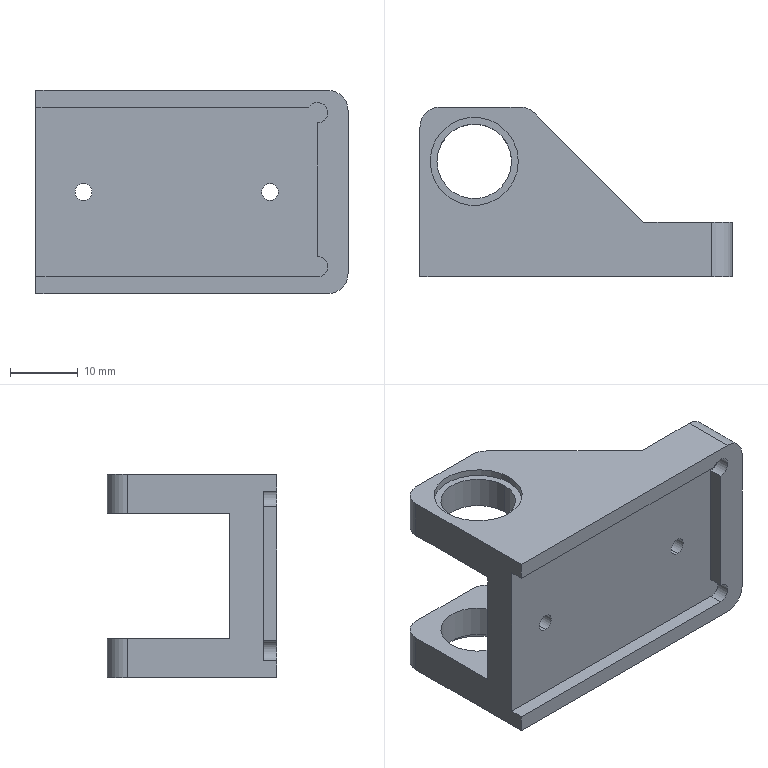Part | NX | features BREP 1 | 1 solid | 43 faces | box 46 x 25 x 30 mm | volume 11465 mm3 | cylinder 22 | plane 21 | commonest cylinder face diameters 6 x6 2.5 x4 11 x4 13 x4 3 x2 8 x2
STEP:
#1=CARTESIAN_POINT('',(26.5,-10.,1.25));
#2=VERTEX_POINT('',#1);
#3=CARTESIAN_POINT('',(26.5,-15.,1.25));
#4=VERTEX_POINT('',#3);
#5=CARTESIAN_POINT('',(26.5,-15.,1.25));
#6=DIRECTION('',(0.,-1.,0.));
#7=VECTOR('',#6,1000.);
#8=LINE('',#5,#7);
#9=EDGE_CURVE('',#2,#4,#8,.T.);
#10=ORIENTED_EDGE('',*,*,#9,.F.);
#11=CARTESIAN_POINT('',(26.5,-10.,-1.25));
#12=VERTEX_POINT('',#11);
#13=CARTESIAN_POINT('',(26.5,-10.,0.));
#14=DIRECTION('',(0.,-1.,0.));
#15=DIRECTION('',(0.,0.,-1.));
#16=AXIS2_PLACEMENT_3D('',#13,#14,#15);
#17=CIRCLE('',#16,1.25);
#18=EDGE_CURVE('',#12,#2,#17,.T.);
#19=ORIENTED_EDGE('',*,*,#18,.F.);
#20=CARTESIAN_POINT('',(26.5,-15.,-1.25));
#21=VERTEX_POINT('',#20);
#22=CARTESIAN_POINT('',(26.5,-15.,-1.25));
#23=DIRECTION('',(0.,-1.,0.));
#24=VECTOR('',#23,1000.);
#25=LINE('',#22,#24);
#26=EDGE_CURVE('',#12,#21,#25,.T.);
#27=ORIENTED_EDGE('',*,*,#26,.T.);
#28=CARTESIAN_POINT('',(26.5,-15.,0.));
#29=DIRECTION('',(0.,-1.,0.));
#30=DIRECTION('',(0.,0.,-1.));
#31=AXIS2_PLACEMENT_3D('',#28,#29,#30);
#32=CIRCLE('',#31,1.25);
#33=EDGE_CURVE('',#21,#4,#32,.T.);
#34=ORIENTED_EDGE('',*,*,#33,.T.);
#35=EDGE_LOOP('',(#10,#19,#27,#34));
#36=FACE_BOUND('',#35,.T.);
#37=CARTESIAN_POINT('',(26.5,-15.,0.));
#38=DIRECTION('',(0.,-1.,0.));
#39=DIRECTION('',(0.,0.,-1.));
#40=AXIS2_PLACEMENT_3D('',#37,#38,#39);
#41=CYLINDRICAL_SURFACE('',#40,1.25);
#42=ADVANCED_FACE('',(#36),#41,.F.);
#43=CARTESIAN_POINT('',(-1.,-10.,1.25));
#44=VERTEX_POINT('',#43);
#45=CARTESIAN_POINT('',(-1.,-15.,1.25));
#46=VERTEX_POINT('',#45);
#47=CARTESIAN_POINT('',(-1.,-15.,1.25));
#48=DIRECTION('',(0.,-1.,0.));
#49=VECTOR('',#48,1000.);
#50=LINE('',#47,#49);
#51=EDGE_CURVE('',#44,#46,#50,.T.);
#52=ORIENTED_EDGE('',*,*,#51,.F.);
#53=CARTESIAN_POINT('',(-1.,-10.,-1.25));
#54=VERTEX_POINT('',#53);
#55=CARTESIAN_POINT('',(-1.,-10.,0.));
#56=DIRECTION('',(0.,-1.,0.));
#57=DIRECTION('',(0.,0.,-1.));
#58=AXIS2_PLACEMENT_3D('',#55,#56,#57);
#59=CIRCLE('',#58,1.25);
#60=EDGE_CURVE('',#54,#44,#59,.T.);
#61=ORIENTED_EDGE('',*,*,#60,.F.);
#62=CARTESIAN_POINT('',(-1.,-15.,-1.25));
#63=VERTEX_POINT('',#62);
#64=CARTESIAN_POINT('',(-1.,-15.,-1.25));
#65=DIRECTION('',(0.,-1.,0.));
#66=VECTOR('',#65,1000.);
#67=LINE('',#64,#66);
#68=EDGE_CURVE('',#54,#63,#67,.T.);
#69=ORIENTED_EDGE('',*,*,#68,.T.);
#70=CARTESIAN_POINT('',(-1.,-15.,0.));
#71=DIRECTION('',(0.,-1.,0.));
#72=DIRECTION('',(0.,0.,-1.));
#73=AXIS2_PLACEMENT_3D('',#70,#71,#72);
#74=CIRCLE('',#73,1.25);
#75=EDGE_CURVE('',#63,#46,#74,.T.);
#76=ORIENTED_EDGE('',*,*,#75,.T.);
#77=EDGE_LOOP('',(#52,#61,#69,#76));
#78=FACE_BOUND('',#77,.T.);
#79=CARTESIAN_POINT('',(-1.,-15.,0.));
#80=DIRECTION('',(0.,-1.,0.));
#81=DIRECTION('',(0.,0.,-1.));
#82=AXIS2_PLACEMENT_3D('',#79,#80,#81);
#83=CYLINDRICAL_SURFACE('',#82,1.25);
#84=ADVANCED_FACE('',(#78),#83,.F.);
#85=CARTESIAN_POINT('',(32.,-13.,4.));
#86=VERTEX_POINT('',#85);
#87=CARTESIAN_POINT('',(32.,-13.,-4.));
#88=VERTEX_POINT('',#87);
#89=CARTESIAN_POINT('',(32.,-13.,0.));
#90=DIRECTION('',(0.,1.,0.));
#91=DIRECTION('',(0.,0.,1.));
#92=AXIS2_PLACEMENT_3D('',#89,#90,#91);
#93=CIRCLE('',#92,4.);
#94=EDGE_CURVE('',#86,#88,#93,.T.);
#95=ORIENTED_EDGE('',*,*,#94,.T.);
#96=CARTESIAN_POINT('',(32.,-13.,0.));
#97=DIRECTION('',(0.,1.,0.));
#98=DIRECTION('',(0.,0.,1.));
#99=AXIS2_PLACEMENT_3D('',#96,#97,#98);
#100=CIRCLE('',#99,4.);
#101=EDGE_CURVE('',#88,#86,#100,.T.);
#102=ORIENTED_EDGE('',*,*,#101,.T.);
#103=EDGE_LOOP('',(#95,#102));
#104=FACE_BOUND('',#103,.T.);
#105=CARTESIAN_POINT('',(32.,-13.,0.));
#106=DIRECTION('',(0.,1.,0.));
#107=DIRECTION('',(0.,0.,1.));
#108=AXIS2_PLACEMENT_3D('',#105,#106,#107);
#109=PLANE('',#108);
#110=ADVANCED_FACE('',(#104),#109,.T.);
#111=CARTESIAN_POINT('',(32.,-10.,-4.));
#112=VERTEX_POINT('',#111);
#113=CARTESIAN_POINT('',(32.,-13.,-4.));
#114=DIRECTION('',(0.,1.,0.));
#115=VECTOR('',#114,1000.);
#116=LINE('',#113,#115);
#117=EDGE_CURVE('',#112,#88,#116,.F.);
#118=ORIENTED_EDGE('',*,*,#117,.T.);
#119=ORIENTED_EDGE('',*,*,#94,.F.);
#120=CARTESIAN_POINT('',(32.,-10.,4.));
#121=VERTEX_POINT('',#120);
#122=CARTESIAN_POINT('',(32.,-13.,4.));
#123=DIRECTION('',(0.,1.,0.));
#124=VECTOR('',#123,1000.);
#125=LINE('',#122,#124);
#126=EDGE_CURVE('',#121,#86,#125,.F.);
#127=ORIENTED_EDGE('',*,*,#126,.F.);
#128=CARTESIAN_POINT('',(32.,-10.,0.));
#129=DIRECTION('',(0.,-1.,0.));
#130=DIRECTION('',(0.,0.,-1.));
#131=AXIS2_PLACEMENT_3D('',#128,#129,#130);
#132=CIRCLE('',#131,4.);
#133=EDGE_CURVE('',#112,#121,#132,.T.);
#134=ORIENTED_EDGE('',*,*,#133,.F.);
#135=EDGE_LOOP('',(#118,#119,#127,#134));
#136=FACE_BOUND('',#135,.T.);
#137=CARTESIAN_POINT('',(32.,-13.,0.));
#138=DIRECTION('',(0.,1.,0.));
#139=DIRECTION('',(0.,0.,1.));
#140=AXIS2_PLACEMENT_3D('',#137,#138,#139);
#141=CYLINDRICAL_SURFACE('',#140,4.);
#142=ADVANCED_FACE('',(#136),#141,.F.);
#143=CARTESIAN_POINT('',(-5.,8.,-9.25));
#144=VERTEX_POINT('',#143);
#145=CARTESIAN_POINT('',(-8.,5.,-9.25));
#146=VERTEX_POINT('',#145);
#147=CARTESIAN_POINT('',(-5.,5.,-9.25));
#148=DIRECTION('',(0.,0.,1.));
#149=DIRECTION('',(0.,1.,0.));
#150=AXIS2_PLACEMENT_3D('',#147,#148,#149);
#151=CIRCLE('',#150,3.);
#152=EDGE_CURVE('',#144,#146,#151,.T.);
#153=ORIENTED_EDGE('',*,*,#152,.F.);
#154=CARTESIAN_POINT('',(-5.,8.,-15.));
#155=VERTEX_POINT('',#154);
#156=CARTESIAN_POINT('',(-5.,8.,15.));
#157=DIRECTION('',(0.,0.,1.));
#158=VECTOR('',#157,1000.);
#159=LINE('',#156,#158);
#160=EDGE_CURVE('',#155,#144,#159,.T.);
#161=ORIENTED_EDGE('',*,*,#160,.F.);
#162=CARTESIAN_POINT('',(-8.,5.,-15.));
#163=VERTEX_POINT('',#162);
#164=CARTESIAN_POINT('',(-5.,5.,-15.));
#165=DIRECTION('',(0.,0.,-1.));
#166=DIRECTION('',(1.,0.,0.));
#167=AXIS2_PLACEMENT_3D('',#164,#165,#166);
#168=CIRCLE('',#167,3.);
#169=EDGE_CURVE('',#163,#155,#168,.T.);
#170=ORIENTED_EDGE('',*,*,#169,.F.);
#171=CARTESIAN_POINT('',(-8.,5.,15.));
#172=DIRECTION('',(0.,0.,-1.));
#173=VECTOR('',#172,1000.);
#174=LINE('',#171,#173);
#175=EDGE_CURVE('',#146,#163,#174,.T.);
#176=ORIENTED_EDGE('',*,*,#175,.F.);
#177=EDGE_LOOP('',(#153,#161,#170,#176));
#178=FACE_BOUND('',#177,.T.);
#179=CARTESIAN_POINT('',(-5.,5.,15.));
#180=DIRECTION('',(0.,0.,-1.));
#181=DIRECTION('',(-1.,0.,0.));
#182=AXIS2_PLACEMENT_3D('',#179,#180,#181);
#183=CYLINDRICAL_SURFACE('',#182,3.);
#184=ADVANCED_FACE('',(#178),#183,.T.);
#185=CARTESIAN_POINT('',(-5.,8.,15.));
#186=VERTEX_POINT('',#185);
#187=CARTESIAN_POINT('',(-8.,5.,15.));
#188=VERTEX_POINT('',#187);
#189=CARTESIAN_POINT('',(-5.,5.,15.));
#190=DIRECTION('',(0.,0.,1.));
#191=DIRECTION('',(1.,0.,0.));
#192=AXIS2_PLACEMENT_3D('',#189,#190,#191);
#193=CIRCLE('',#192,3.);
#194=EDGE_CURVE('',#186,#188,#193,.T.);
#195=ORIENTED_EDGE('',*,*,#194,.F.);
#196=CARTESIAN_POINT('',(-5.,8.,9.25));
#197=VERTEX_POINT('',#196);
#198=CARTESIAN_POINT('',(-5.,8.,15.));
#199=DIRECTION('',(0.,0.,1.));
#200=VECTOR('',#199,1000.);
#201=LINE('',#198,#200);
#202=EDGE_CURVE('',#197,#186,#201,.T.);
#203=ORIENTED_EDGE('',*,*,#202,.F.);
#204=CARTESIAN_POINT('',(-8.,5.,9.25));
#205=VERTEX_POINT('',#204);
#206=CARTESIAN_POINT('',(-5.,5.,9.25));
#207=DIRECTION('',(0.,0.,-1.));
#208=DIRECTION('',(0.,-1.,0.));
#209=AXIS2_PLACEMENT_3D('',#206,#207,#208);
#210=CIRCLE('',#209,3.);
#211=EDGE_CURVE('',#205,#197,#210,.T.);
#212=ORIENTED_EDGE('',*,*,#211,.F.);
#213=CARTESIAN_POINT('',(-8.,5.,15.));
#214=DIRECTION('',(0.,0.,-1.));
#215=VECTOR('',#214,1000.);
#216=LINE('',#213,#215);
#217=EDGE_CURVE('',#188,#205,#216,.T.);
#218=ORIENTED_EDGE('',*,*,#217,.F.);
#219=EDGE_LOOP('',(#195,#203,#212,#218));
#220=FACE_BOUND('',#219,.T.);
#221=CARTESIAN_POINT('',(-5.,5.,15.));
#222=DIRECTION('',(0.,0.,-1.));
#223=DIRECTION('',(-1.,0.,0.));
#224=AXIS2_PLACEMENT_3D('',#221,#222,#223);
#225=CYLINDRICAL_SURFACE('',#224,3.);
#226=ADVANCED_FACE('',(#220),#225,.T.);
#227=CARTESIAN_POINT('',(8.879,7.121,-9.25));
#228=VERTEX_POINT('',#227);
#229=CARTESIAN_POINT('',(6.757,8.,-9.25));
#230=VERTEX_POINT('',#229);
#231=CARTESIAN_POINT('',(6.757,5.,-9.25));
#232=DIRECTION('',(0.,0.,1.));
#233=DIRECTION('',(0.,1.,0.));
#234=AXIS2_PLACEMENT_3D('',#231,#232,#233);
#235=CIRCLE('',#234,3.);
#236=EDGE_CURVE('',#228,#230,#235,.T.);
#237=ORIENTED_EDGE('',*,*,#236,.F.);
#238=CARTESIAN_POINT('',(8.879,7.121,-15.));
#239=VERTEX_POINT('',#238);
#240=CARTESIAN_POINT('',(8.879,7.121,15.));
#241=DIRECTION('',(0.,0.,1.));
#242=VECTOR('',#241,1000.);
#243=LINE('',#240,#242);
#244=EDGE_CURVE('',#239,#228,#243,.T.);
#245=ORIENTED_EDGE('',*,*,#244,.F.);
#246=CARTESIAN_POINT('',(6.757,8.,-15.));
#247=VERTEX_POINT('',#246);
#248=CARTESIAN_POINT('',(6.757,5.,-15.));
#249=DIRECTION('',(0.,0.,-1.));
#250=DIRECTION('',(1.,0.,0.));
#251=AXIS2_PLACEMENT_3D('',#248,#249,#250);
#252=CIRCLE('',#251,3.);
#253=EDGE_CURVE('',#247,#239,#252,.T.);
#254=ORIENTED_EDGE('',*,*,#253,.F.);
#255=CARTESIAN_POINT('',(6.757,8.,15.));
#256=DIRECTION('',(0.,0.,-1.));
#257=VECTOR('',#256,1000.);
#258=LINE('',#255,#257);
#259=EDGE_CURVE('',#230,#247,#258,.T.);
#260=ORIENTED_EDGE('',*,*,#259,.F.);
#261=EDGE_LOOP('',(#237,#245,#254,#260));
#262=FACE_BOUND('',#261,.T.);
#263=CARTESIAN_POINT('',(6.757,5.,15.));
#264=DIRECTION('',(0.,0.,-1.));
#265=DIRECTION('',(-1.,0.,0.));
#266=AXIS2_PLACEMENT_3D('',#263,#264,#265);
#267=CYLINDRICAL_SURFACE('',#266,3.);
#268=ADVANCED_FACE('',(#262),#267,.T.);
#269=CARTESIAN_POINT('',(8.879,7.121,15.));
#270=VERTEX_POINT('',#269);
#271=CARTESIAN_POINT('',(6.757,8.,15.));
#272=VERTEX_POINT('',#271);
#273=CARTESIAN_POINT('',(6.757,5.,15.));
#274=DIRECTION('',(0.,0.,1.));
#275=DIRECTION('',(1.,0.,0.));
#276=AXIS2_PLACEMENT_3D('',#273,#274,#275);
#277=CIRCLE('',#276,3.);
#278=EDGE_CURVE('',#270,#272,#277,.T.);
#279=ORIENTED_EDGE('',*,*,#278,.F.);
#280=CARTESIAN_POINT('',(8.879,7.121,9.25));
#281=VERTEX_POINT('',#280);
#282=CARTESIAN_POINT('',(8.879,7.121,15.));
#283=DIRECTION('',(0.,0.,1.));
#284=VECTOR('',#283,1000.);
#285=LINE('',#282,#284);
#286=EDGE_CURVE('',#281,#270,#285,.T.);
#287=ORIENTED_EDGE('',*,*,#286,.F.);
#288=CARTESIAN_POINT('',(6.757,8.,9.25));
#289=VERTEX_POINT('',#288);
#290=CARTESIAN_POINT('',(6.757,5.,9.25));
#291=DIRECTION('',(0.,0.,-1.));
#292=DIRECTION('',(0.,-1.,0.));
#293=AXIS2_PLACEMENT_3D('',#290,#291,#292);
#294=CIRCLE('',#293,3.);
#295=EDGE_CURVE('',#289,#281,#294,.T.);
#296=ORIENTED_EDGE('',*,*,#295,.F.);
#297=CARTESIAN_POINT('',(6.757,8.,15.));
#298=DIRECTION('',(0.,0.,-1.));
#299=VECTOR('',#298,1000.);
#300=LINE('',#297,#299);
#301=EDGE_CURVE('',#272,#289,#300,.T.);
#302=ORIENTED_EDGE('',*,*,#301,.F.);
#303=EDGE_LOOP('',(#279,#287,#296,#302));
#304=FACE_BOUND('',#303,.T.);
#305=CARTESIAN_POINT('',(6.757,5.,15.));
#306=DIRECTION('',(0.,0.,-1.));
#307=DIRECTION('',(-1.,0.,0.));
#308=AXIS2_PLACEMENT_3D('',#305,#306,#307);
#309=CYLINDRICAL_SURFACE('',#308,3.);
#310=ADVANCED_FACE('',(#304),#309,.T.);
#311=CARTESIAN_POINT('',(38.,-17.,12.));
#312=VERTEX_POINT('',#311);
#313=CARTESIAN_POINT('',(35.,-17.,15.));
#314=VERTEX_POINT('',#313);
#315=CARTESIAN_POINT('',(35.,-17.,12.));
#316=DIRECTION('',(0.,-1.,0.));
#317=DIRECTION('',(0.,0.,1.));
#318=AXIS2_PLACEMENT_3D('',#315,#316,#317);
#319=CIRCLE('',#318,3.);
#320=EDGE_CURVE('',#312,#314,#319,.T.);
#321=ORIENTED_EDGE('',*,*,#320,.F.);
#322=CARTESIAN_POINT('',(38.,-9.,12.));
#323=VERTEX_POINT('',#322);
#324=CARTESIAN_POINT('',(38.,-17.,12.));
#325=DIRECTION('',(0.,-1.,0.));
#326=VECTOR('',#325,1000.);
#327=LINE('',#324,#326);
#328=EDGE_CURVE('',#323,#312,#327,.T.);
#329=ORIENTED_EDGE('',*,*,#328,.F.);
#330=CARTESIAN_POINT('',(35.,-9.,15.));
#331=VERTEX_POINT('',#330);
#332=CARTESIAN_POINT('',(35.,-9.,12.));
#333=DIRECTION('',(0.,1.,0.));
#334=DIRECTION('',(0.,0.,-1.));
#335=AXIS2_PLACEMENT_3D('',#332,#333,#334);
#336=CIRCLE('',#335,3.);
#337=EDGE_CURVE('',#331,#323,#336,.T.);
#338=ORIENTED_EDGE('',*,*,#337,.F.);
#339=CARTESIAN_POINT('',(35.,-9.,15.));
#340=DIRECTION('',(0.,1.,0.));
#341=VECTOR('',#340,1000.);
#342=LINE('',#339,#341);
#343=EDGE_CURVE('',#314,#331,#342,.T.);
#344=ORIENTED_EDGE('',*,*,#343,.F.);
#345=EDGE_LOOP('',(#321,#329,#338,#344));
#346=FACE_BOUND('',#345,.T.);
#347=CARTESIAN_POINT('',(35.,0.,12.));
#348=DIRECTION('',(0.,-1.,0.));
#349=DIRECTION('',(0.,0.,-1.));
#350=AXIS2_PLACEMENT_3D('',#347,#348,#349);
#351=CYLINDRICAL_SURFACE('',#350,3.);
#352=ADVANCED_FACE('',(#346),#351,.T.);
#353=CARTESIAN_POINT('',(35.,-17.,-15.));
#354=VERTEX_POINT('',#353);
#355=CARTESIAN_POINT('',(38.,-17.,-12.));
#356=VERTEX_POINT('',#355);
#357=CARTESIAN_POINT('',(35.,-17.,-12.));
#358=DIRECTION('',(0.,-1.,0.));
#359=DIRECTION('',(0.,0.,1.));
#360=AXIS2_PLACEMENT_3D('',#357,#358,#359);
#361=CIRCLE('',#360,3.);
#362=EDGE_CURVE('',#354,#356,#361,.T.);
#363=ORIENTED_EDGE('',*,*,#362,.F.);
#364=CARTESIAN_POINT('',(35.,-9.,-15.));
#365=VERTEX_POINT('',#364);
#366=CARTESIAN_POINT('',(35.,0.,-15.));
#367=DIRECTION('',(0.,-1.,0.));
#368=VECTOR('',#367,1000.);
#369=LINE('',#366,#368);
#370=EDGE_CURVE('',#365,#354,#369,.T.);
#371=ORIENTED_EDGE('',*,*,#370,.F.);
#372=CARTESIAN_POINT('',(38.,-9.,-12.));
#373=VERTEX_POINT('',#372);
#374=CARTESIAN_POINT('',(35.,-9.,-12.));
#375=DIRECTION('',(0.,1.,0.));
#376=DIRECTION('',(0.,0.,-1.));
#377=AXIS2_PLACEMENT_3D('',#374,#375,#376);
#378=CIRCLE('',#377,3.);
#379=EDGE_CURVE('',#373,#365,#378,.T.);
#380=ORIENTED_EDGE('',*,*,#379,.F.);
#381=CARTESIAN_POINT('',(38.,-9.,-12.));
#382=DIRECTION('',(0.,1.,0.));
#383=VECTOR('',#382,1000.);
#384=LINE('',#381,#383);
#385=EDGE_CURVE('',#356,#373,#384,.T.);
#386=ORIENTED_EDGE('',*,*,#385,.F.);
#387=EDGE_LOOP('',(#363,#371,#380,#386));
#388=FACE_BOUND('',#387,.T.);
#389=CARTESIAN_POINT('',(35.,-9.,-12.));
#390=DIRECTION('',(0.,1.,0.));
#391=DIRECTION('',(0.,0.,1.));
#392=AXIS2_PLACEMENT_3D('',#389,#390,#391);
#393=CYLINDRICAL_SURFACE('',#392,3.);
#394=ADVANCED_FACE('',(#388),#393,.T.);
#395=CARTESIAN_POINT('',(-8.,-15.,12.5));
#396=VERTEX_POINT('',#395);
#397=CARTESIAN_POINT('',(-8.,-15.,-12.5));
#398=VERTEX_POINT('',#397);
#399=CARTESIAN_POINT('',(-8.,-15.,12.5));
#400=DIRECTION('',(0.,0.,-1.));
#401=VECTOR('',#400,1000.);
#402=LINE('',#399,#401);
#403=EDGE_CURVE('',#396,#398,#402,.T.);
#404=ORIENTED_EDGE('',*,*,#403,.T.);
#405=CARTESIAN_POINT('',(33.5,-15.,-12.5));
#406=VERTEX_POINT('',#405);
#407=CARTESIAN_POINT('',(33.5,-15.,-12.5));
#408=DIRECTION('',(1.,0.,0.));
#409=VECTOR('',#408,1000.);
#410=LINE('',#407,#409);
#411=EDGE_CURVE('',#398,#406,#410,.T.);
#412=ORIENTED_EDGE('',*,*,#411,.T.);
#413=CARTESIAN_POINT('',(33.5,-15.,-9.5));
#414=VERTEX_POINT('',#413);
#415=CARTESIAN_POINT('',(33.5,-15.,-11.));
#416=DIRECTION('',(0.,-1.,0.));
#417=DIRECTION('',(0.,0.,-1.));
#418=AXIS2_PLACEMENT_3D('',#415,#416,#417);
#419=CIRCLE('',#418,1.5);
#420=EDGE_CURVE('',#406,#414,#419,.T.);
#421=ORIENTED_EDGE('',*,*,#420,.T.);
#422=CARTESIAN_POINT('',(33.5,-15.,10.202));
#423=VERTEX_POINT('',#422);
#424=CARTESIAN_POINT('',(33.5,-15.,10.202));
#425=DIRECTION('',(0.,0.,1.));
#426=VECTOR('',#425,1000.);
#427=LINE('',#424,#426);
#428=EDGE_CURVE('',#414,#423,#427,.T.);
#429=ORIENTED_EDGE('',*,*,#428,.T.);
#430=CARTESIAN_POINT('',(32.23,-15.,12.5));
#431=VERTEX_POINT('',#430);
#432=CARTESIAN_POINT('',(33.5,-15.,11.702));
#433=DIRECTION('',(0.,-1.,0.));
#434=DIRECTION('',(0.,0.,-1.));
#435=AXIS2_PLACEMENT_3D('',#432,#433,#434);
#436=CIRCLE('',#435,1.5);
#437=EDGE_CURVE('',#423,#431,#436,.T.);
#438=ORIENTED_EDGE('',*,*,#437,.T.);
#439=CARTESIAN_POINT('',(32.23,-15.,12.5));
#440=DIRECTION('',(-1.,0.,0.));
#441=VECTOR('',#440,1000.);
#442=LINE('',#439,#441);
#443=EDGE_CURVE('',#431,#396,#442,.T.);
#444=ORIENTED_EDGE('',*,*,#443,.T.);
#445=EDGE_LOOP('',(#404,#412,#421,#429,#438,#444));
#446=FACE_BOUND('',#445,.T.);
#447=ORIENTED_EDGE('',*,*,#75,.F.);
#448=CARTESIAN_POINT('',(-1.,-15.,0.));
#449=DIRECTION('',(0.,-1.,0.));
#450=DIRECTION('',(0.,0.,-1.));
#451=AXIS2_PLACEMENT_3D('',#448,#449,#450);
#452=CIRCLE('',#451,1.25);
#453=EDGE_CURVE('',#46,#63,#452,.T.);
#454=ORIENTED_EDGE('',*,*,#453,.F.);
#455=EDGE_LOOP('',(#447,#454));
#456=FACE_BOUND('',#455,.T.);
#457=ORIENTED_EDGE('',*,*,#33,.F.);
#458=CARTESIAN_POINT('',(26.5,-15.,0.));
#459=DIRECTION('',(0.,-1.,0.));
#460=DIRECTION('',(0.,0.,-1.));
#461=AXIS2_PLACEMENT_3D('',#458,#459,#460);
#462=CIRCLE('',#461,1.25);
#463=EDGE_CURVE('',#4,#21,#462,.T.);
#464=ORIENTED_EDGE('',*,*,#463,.F.);
#465=EDGE_LOOP('',(#457,#464));
#466=FACE_BOUND('',#465,.T.);
#467=CARTESIAN_POINT('',(33.5,-15.,-11.));
#468=DIRECTION('',(0.,-1.,0.));
#469=DIRECTION('',(0.,0.,-1.));
#470=AXIS2_PLACEMENT_3D('',#467,#468,#469);
#471=PLANE('',#470);
#472=ADVANCED_FACE('',(#446,#456,#466),#471,.T.);
#473=CARTESIAN_POINT('',(-8.,-17.,-12.5));
#474=VERTEX_POINT('',#473);
#475=CARTESIAN_POINT('',(33.5,-17.,-12.5));
#476=VERTEX_POINT('',#475);
#477=CARTESIAN_POINT('',(33.5,-17.,-12.5));
#478=DIRECTION('',(1.,0.,0.));
#479=VECTOR('',#478,1000.);
#480=LINE('',#477,#479);
#481=EDGE_CURVE('',#474,#476,#480,.T.);
#482=ORIENTED_EDGE('',*,*,#481,.T.);
#483=CARTESIAN_POINT('',(33.5,-15.,-12.5));
#484=DIRECTION('',(0.,-1.,0.));
#485=VECTOR('',#484,1000.);
#486=LINE('',#483,#485);
#487=EDGE_CURVE('',#406,#476,#486,.T.);
#488=ORIENTED_EDGE('',*,*,#487,.F.);
#489=ORIENTED_EDGE('',*,*,#411,.F.);
#490=CARTESIAN_POINT('',(-8.,-15.,-12.5));
#491=DIRECTION('',(0.,-1.,0.));
#492=VECTOR('',#491,1000.);
#493=LINE('',#490,#492);
#494=EDGE_CURVE('',#398,#474,#493,.T.);
#495=ORIENTED_EDGE('',*,*,#494,.T.);
#496=EDGE_LOOP('',(#482,#488,#489,#495));
#497=FACE_BOUND('',#496,.T.);
#498=CARTESIAN_POINT('',(33.5,-15.,-12.5));
#499=DIRECTION('',(0.,0.,-1.));
#500=DIRECTION('',(-1.,0.,0.));
#501=AXIS2_PLACEMENT_3D('',#498,#499,#500);
#502=PLANE('',#501);
#503=ADVANCED_FACE('',(#497),#502,.F.);
#504=CARTESIAN_POINT('',(33.5,-17.,-9.5));
#505=VERTEX_POINT('',#504);
#506=CARTESIAN_POINT('',(33.5,-17.,-11.));
#507=DIRECTION('',(0.,-1.,0.));
#508=DIRECTION('',(0.,0.,-1.));
#509=AXIS2_PLACEMENT_3D('',#506,#507,#508);
#510=CIRCLE('',#509,1.5);
#511=EDGE_CURVE('',#476,#505,#510,.T.);
#512=ORIENTED_EDGE('',*,*,#511,.T.);
#513=CARTESIAN_POINT('',(33.5,-15.,-9.5));
#514=DIRECTION('',(0.,-1.,0.));
#515=VECTOR('',#514,1000.);
#516=LINE('',#513,#515);
#517=EDGE_CURVE('',#414,#505,#516,.T.);
#518=ORIENTED_EDGE('',*,*,#517,.F.);
#519=ORIENTED_EDGE('',*,*,#420,.F.);
#520=ORIENTED_EDGE('',*,*,#487,.T.);
#521=EDGE_LOOP('',(#512,#518,#519,#520));
#522=FACE_BOUND('',#521,.T.);
#523=CARTESIAN_POINT('',(33.5,-15.,-11.));
#524=DIRECTION('',(0.,-1.,0.));
#525=DIRECTION('',(0.,0.,-1.));
#526=AXIS2_PLACEMENT_3D('',#523,#524,#525);
#527=CYLINDRICAL_SURFACE('',#526,1.5);
#528=ADVANCED_FACE('',(#522),#527,.F.);
#529=CARTESIAN_POINT('',(33.5,-17.,10.202));
#530=VERTEX_POINT('',#529);
#531=CARTESIAN_POINT('',(33.5,-17.,10.202));
#532=DIRECTION('',(0.,0.,1.));
#533=VECTOR('',#532,1000.);
#534=LINE('',#531,#533);
#535=EDGE_CURVE('',#505,#530,#534,.T.);
#536=ORIENTED_EDGE('',*,*,#535,.T.);
#537=CARTESIAN_POINT('',(33.5,-15.,10.202));
#538=DIRECTION('',(0.,-1.,0.));
#539=VECTOR('',#538,1000.);
#540=LINE('',#537,#539);
#541=EDGE_CURVE('',#423,#530,#540,.T.);
#542=ORIENTED_EDGE('',*,*,#541,.F.);
#543=ORIENTED_EDGE('',*,*,#428,.F.);
#544=ORIENTED_EDGE('',*,*,#517,.T.);
#545=EDGE_LOOP('',(#536,#542,#543,#544));
#546=FACE_BOUND('',#545,.T.);
#547=CARTESIAN_POINT('',(33.5,-15.,10.202));
#548=DIRECTION('',(1.,0.,0.));
#549=DIRECTION('',(0.,0.,-1.));
#550=AXIS2_PLACEMENT_3D('',#547,#548,#549);
#551=PLANE('',#550);
#552=ADVANCED_FACE('',(#546),#551,.F.);
#553=CARTESIAN_POINT('',(32.23,-17.,12.5));
#554=VERTEX_POINT('',#553);
#555=CARTESIAN_POINT('',(33.5,-17.,11.702));
#556=DIRECTION('',(0.,-1.,0.));
#557=DIRECTION('',(0.,0.,-1.));
#558=AXIS2_PLACEMENT_3D('',#555,#556,#557);
#559=CIRCLE('',#558,1.5);
#560=EDGE_CURVE('',#530,#554,#559,.T.);
#561=ORIENTED_EDGE('',*,*,#560,.T.);
#562=CARTESIAN_POINT('',(32.23,-15.,12.5));
#563=DIRECTION('',(0.,-1.,0.));
#564=VECTOR('',#563,1000.);
#565=LINE('',#562,#564);
#566=EDGE_CURVE('',#431,#554,#565,.T.);
#567=ORIENTED_EDGE('',*,*,#566,.F.);
#568=ORIENTED_EDGE('',*,*,#437,.F.);
#569=ORIENTED_EDGE('',*,*,#541,.T.);
#570=EDGE_LOOP('',(#561,#567,#568,#569));
#571=FACE_BOUND('',#570,.T.);
#572=CARTESIAN_POINT('',(33.5,-15.,11.702));
#573=DIRECTION('',(0.,-1.,0.));
#574=DIRECTION('',(0.,0.,-1.));
#575=AXIS2_PLACEMENT_3D('',#572,#573,#574);
#576=CYLINDRICAL_SURFACE('',#575,1.5);
#577=ADVANCED_FACE('',(#571),#576,.F.);
#578=CARTESIAN_POINT('',(-8.,-17.,12.5));
#579=VERTEX_POINT('',#578);
#580=CARTESIAN_POINT('',(32.23,-17.,12.5));
#581=DIRECTION('',(-1.,0.,0.));
#582=VECTOR('',#581,1000.);
#583=LINE('',#580,#582);
#584=EDGE_CURVE('',#554,#579,#583,.T.);
#585=ORIENTED_EDGE('',*,*,#584,.T.);
#586=CARTESIAN_POINT('',(-8.,-15.,12.5));
#587=DIRECTION('',(0.,-1.,0.));
#588=VECTOR('',#587,1000.);
#589=LINE('',#586,#588);
#590=EDGE_CURVE('',#396,#579,#589,.T.);
#591=ORIENTED_EDGE('',*,*,#590,.F.);
#592=ORIENTED_EDGE('',*,*,#443,.F.);
#593=ORIENTED_EDGE('',*,*,#566,.T.);
#594=EDGE_LOOP('',(#585,#591,#592,#593));
#595=FACE_BOUND('',#594,.T.);
#596=CARTESIAN_POINT('',(32.23,-15.,12.5));
#597=DIRECTION('',(0.,0.,1.));
#598=DIRECTION('',(1.,0.,0.));
#599=AXIS2_PLACEMENT_3D('',#596,#597,#598);
#600=PLANE('',#599);
#601=ADVANCED_FACE('',(#595),#600,.F.);
#602=CARTESIAN_POINT('',(-6.5,0.,-14.));
#603=VERTEX_POINT('',#602);
#604=CARTESIAN_POINT('',(6.5,0.,-14.));
#605=VERTEX_POINT('',#604);
#606=CARTESIAN_POINT('',(0.,0.,-14.));
#607=DIRECTION('',(0.,0.,-1.));
#608=DIRECTION('',(-1.,0.,0.));
#609=AXIS2_PLACEMENT_3D('',#606,#607,#608);
#610=CIRCLE('',#609,6.5);
#611=EDGE_CURVE('',#603,#605,#610,.T.);
#612=ORIENTED_EDGE('',*,*,#611,.T.);
#613=CARTESIAN_POINT('',(0.,0.,-14.));
#614=DIRECTION('',(0.,0.,-1.));
#615=DIRECTION('',(-1.,0.,0.));
#616=AXIS2_PLACEMENT_3D('',#613,#614,#615);
#617=CIRCLE('',#616,6.5);
#618=EDGE_CURVE('',#605,#603,#617,.T.);
#619=ORIENTED_EDGE('',*,*,#618,.T.);
#620=EDGE_LOOP('',(#612,#619));
#621=FACE_BOUND('',#620,.T.);
#622=CARTESIAN_POINT('',(-5.5,0.,-14.));
#623=VERTEX_POINT('',#622);
#624=CARTESIAN_POINT('',(5.5,0.,-14.));
#625=VERTEX_POINT('',#624);
#626=CARTESIAN_POINT('',(0.,0.,-14.));
#627=DIRECTION('',(0.,0.,-1.));
#628=DIRECTION('',(-1.,0.,0.));
#629=AXIS2_PLACEMENT_3D('',#626,#627,#628);
#630=CIRCLE('',#629,5.5);
#631=EDGE_CURVE('',#623,#625,#630,.T.);
#632=ORIENTED_EDGE('',*,*,#631,.F.);
#633=CARTESIAN_POINT('',(0.,0.,-14.));
#634=DIRECTION('',(0.,0.,-1.));
#635=DIRECTION('',(-1.,0.,0.));
#636=AXIS2_PLACEMENT_3D('',#633,#634,#635);
#637=CIRCLE('',#636,5.5);
#638=EDGE_CURVE('',#625,#623,#637,.T.);
#639=ORIENTED_EDGE('',*,*,#638,.F.);
#640=EDGE_LOOP('',(#632,#639));
#641=FACE_BOUND('',#640,.T.);
#642=CARTESIAN_POINT('',(0.,0.,-14.));
#643=DIRECTION('',(0.,0.,-1.));
#644=DIRECTION('',(-1.,0.,0.));
#645=AXIS2_PLACEMENT_3D('',#642,#643,#644);
#646=PLANE('',#645);
#647=ADVANCED_FACE('',(#621,#641),#646,.T.);
#648=CARTESIAN_POINT('',(6.5,0.,-15.));
#649=VERTEX_POINT('',#648);
#650=CARTESIAN_POINT('',(6.5,0.,-14.));
#651=DIRECTION('',(0.,0.,-1.));
#652=VECTOR('',#651,1000.);
#653=LINE('',#650,#652);
#654=EDGE_CURVE('',#605,#649,#653,.T.);
#655=ORIENTED_EDGE('',*,*,#654,.F.);
#656=ORIENTED_EDGE('',*,*,#611,.F.);
#657=CARTESIAN_POINT('',(-6.5,0.,-15.));
#658=VERTEX_POINT('',#657);
#659=CARTESIAN_POINT('',(-6.5,0.,-14.));
#660=DIRECTION('',(0.,0.,-1.));
#661=VECTOR('',#660,1000.);
#662=LINE('',#659,#661);
#663=EDGE_CURVE('',#603,#658,#662,.T.);
#664=ORIENTED_EDGE('',*,*,#663,.T.);
#665=CARTESIAN_POINT('',(0.,0.,-15.));
#666=DIRECTION('',(0.,0.,-1.));
#667=DIRECTION('',(-1.,0.,0.));
#668=AXIS2_PLACEMENT_3D('',#665,#666,#667);
#669=CIRCLE('',#668,6.5);
#670=EDGE_CURVE('',#658,#649,#669,.T.);
#671=ORIENTED_EDGE('',*,*,#670,.T.);
#672=EDGE_LOOP('',(#655,#656,#664,#671));
#673=FACE_BOUND('',#672,.T.);
#674=CARTESIAN_POINT('',(0.,0.,-14.));
#675=DIRECTION('',(0.,0.,-1.));
#676=DIRECTION('',(-1.,0.,0.));
#677=AXIS2_PLACEMENT_3D('',#674,#675,#676);
#678=CYLINDRICAL_SURFACE('',#677,6.5);
#679=ADVANCED_FACE('',(#673),#678,.F.);
#680=CARTESIAN_POINT('',(6.5,0.,14.));
#681=VERTEX_POINT('',#680);
#682=CARTESIAN_POINT('',(-6.5,0.,14.));
#683=VERTEX_POINT('',#682);
#684=CARTESIAN_POINT('',(0.,0.,14.));
#685=DIRECTION('',(0.,0.,1.));
#686=DIRECTION('',(1.,0.,0.));
#687=AXIS2_PLACEMENT_3D('',#684,#685,#686);
#688=CIRCLE('',#687,6.5);
#689=EDGE_CURVE('',#681,#683,#688,.T.);
#690=ORIENTED_EDGE('',*,*,#689,.T.);
#691=CARTESIAN_POINT('',(0.,0.,14.));
#692=DIRECTION('',(0.,0.,1.));
#693=DIRECTION('',(1.,0.,0.));
#694=AXIS2_PLACEMENT_3D('',#691,#692,#693);
#695=CIRCLE('',#694,6.5);
#696=EDGE_CURVE('',#683,#681,#695,.T.);
#697=ORIENTED_EDGE('',*,*,#696,.T.);
#698=EDGE_LOOP('',(#690,#697));
#699=FACE_BOUND('',#698,.T.);
#700=CARTESIAN_POINT('',(-5.5,0.,14.));
#701=VERTEX_POINT('',#700);
#702=CARTESIAN_POINT('',(5.5,0.,14.));
#703=VERTEX_POINT('',#702);
#704=CARTESIAN_POINT('',(0.,0.,14.));
#705=DIRECTION('',(0.,0.,1.));
#706=DIRECTION('',(1.,0.,0.));
#707=AXIS2_PLACEMENT_3D('',#704,#705,#706);
#708=CIRCLE('',#707,5.5);
#709=EDGE_CURVE('',#701,#703,#708,.T.);
#710=ORIENTED_EDGE('',*,*,#709,.F.);
#711=CARTESIAN_POINT('',(0.,0.,14.));
#712=DIRECTION('',(0.,0.,1.));
#713=DIRECTION('',(1.,0.,0.));
#714=AXIS2_PLACEMENT_3D('',#711,#712,#713);
#715=CIRCLE('',#714,5.5);
#716=EDGE_CURVE('',#703,#701,#715,.T.);
#717=ORIENTED_EDGE('',*,*,#716,.F.);
#718=EDGE_LOOP('',(#710,#717));
#719=FACE_BOUND('',#718,.T.);
#720=CARTESIAN_POINT('',(0.,0.,14.));
#721=DIRECTION('',(0.,0.,1.));
#722=DIRECTION('',(1.,0.,0.));
#723=AXIS2_PLACEMENT_3D('',#720,#721,#722);
#724=PLANE('',#723);
#725=ADVANCED_FACE('',(#699,#719),#724,.T.);
#726=CARTESIAN_POINT('',(-6.5,0.,15.));
#727=VERTEX_POINT('',#726);
#728=CARTESIAN_POINT('',(-6.5,0.,14.));
#729=DIRECTION('',(0.,0.,1.));
#730=VECTOR('',#729,1000.);
#731=LINE('',#728,#730);
#732=EDGE_CURVE('',#727,#683,#731,.F.);
#733=ORIENTED_EDGE('',*,*,#732,.T.);
#734=ORIENTED_EDGE('',*,*,#689,.F.);
#735=CARTESIAN_POINT('',(6.5,0.,15.));
#736=VERTEX_POINT('',#735);
#737=CARTESIAN_POINT('',(6.5,0.,14.));
#738=DIRECTION('',(0.,0.,1.));
#739=VECTOR('',#738,1000.);
#740=LINE('',#737,#739);
#741=EDGE_CURVE('',#736,#681,#740,.F.);
#742=ORIENTED_EDGE('',*,*,#741,.F.);
#743=CARTESIAN_POINT('',(0.,0.,15.));
#744=DIRECTION('',(0.,0.,1.));
#745=DIRECTION('',(1.,0.,0.));
#746=AXIS2_PLACEMENT_3D('',#743,#744,#745);
#747=CIRCLE('',#746,6.5);
#748=EDGE_CURVE('',#736,#727,#747,.T.);
#749=ORIENTED_EDGE('',*,*,#748,.T.);
#750=EDGE_LOOP('',(#733,#734,#742,#749));
#751=FACE_BOUND('',#750,.T.);
#752=CARTESIAN_POINT('',(0.,0.,14.));
#753=DIRECTION('',(0.,0.,1.));
#754=DIRECTION('',(1.,0.,0.));
#755=AXIS2_PLACEMENT_3D('',#752,#753,#754);
#756=CYLINDRICAL_SURFACE('',#755,6.5);
#757=ADVANCED_FACE('',(#751),#756,.F.);
#758=CARTESIAN_POINT('',(-8.,-10.,-9.25));
#759=VERTEX_POINT('',#758);
#760=CARTESIAN_POINT('',(-8.,-10.,9.25));
#761=VERTEX_POINT('',#760);
#762=CARTESIAN_POINT('',(-8.,-10.,-9.25));
#763=DIRECTION('',(0.,0.,1.));
#764=VECTOR('',#763,1000.);
#765=LINE('',#762,#764);
#766=EDGE_CURVE('',#759,#761,#765,.T.);
#767=ORIENTED_EDGE('',*,*,#766,.T.);
#768=CARTESIAN_POINT('',(38.,-10.,9.25));
#769=VERTEX_POINT('',#768);
#770=CARTESIAN_POINT('',(38.,-10.,9.25));
#771=DIRECTION('',(-1.,0.,0.));
#772=VECTOR('',#771,1000.);
#773=LINE('',#770,#772);
#774=EDGE_CURVE('',#769,#761,#773,.T.);
#775=ORIENTED_EDGE('',*,*,#774,.F.);
#776=CARTESIAN_POINT('',(38.,-10.,-9.25));
#777=VERTEX_POINT('',#776);
#778=CARTESIAN_POINT('',(38.,-10.,-9.25));
#779=DIRECTION('',(0.,0.,1.));
#780=VECTOR('',#779,1000.);
#781=LINE('',#778,#780);
#782=EDGE_CURVE('',#777,#769,#781,.T.);
#783=ORIENTED_EDGE('',*,*,#782,.F.);
#784=CARTESIAN_POINT('',(38.,-10.,-9.25));
#785=DIRECTION('',(-1.,0.,0.));
#786=VECTOR('',#785,1000.);
#787=LINE('',#784,#786);
#788=EDGE_CURVE('',#777,#759,#787,.T.);
#789=ORIENTED_EDGE('',*,*,#788,.T.);
#790=EDGE_LOOP('',(#767,#775,#783,#789));
#791=FACE_BOUND('',#790,.T.);
#792=CARTESIAN_POINT('',(32.,-10.,0.));
#793=DIRECTION('',(0.,-1.,0.));
#794=DIRECTION('',(0.,0.,-1.));
#795=AXIS2_PLACEMENT_3D('',#792,#793,#794);
#796=CIRCLE('',#795,4.);
#797=EDGE_CURVE('',#121,#112,#796,.T.);
#798=ORIENTED_EDGE('',*,*,#797,.T.);
#799=ORIENTED_EDGE('',*,*,#133,.T.);
#800=EDGE_LOOP('',(#798,#799));
#801=FACE_BOUND('',#800,.T.);
#802=ORIENTED_EDGE('',*,*,#60,.T.);
#803=CARTESIAN_POINT('',(-1.,-10.,0.));
#804=DIRECTION('',(0.,-1.,0.));
#805=DIRECTION('',(0.,0.,-1.));
#806=AXIS2_PLACEMENT_3D('',#803,#804,#805);
#807=CIRCLE('',#806,1.25);
#808=EDGE_CURVE('',#44,#54,#807,.T.);
#809=ORIENTED_EDGE('',*,*,#808,.T.);
#810=EDGE_LOOP('',(#802,#809));
#811=FACE_BOUND('',#810,.T.);
#812=ORIENTED_EDGE('',*,*,#18,.T.);
#813=CARTESIAN_POINT('',(26.5,-10.,0.));
#814=DIRECTION('',(0.,-1.,0.));
#815=DIRECTION('',(0.,0.,-1.));
#816=AXIS2_PLACEMENT_3D('',#813,#814,#815);
#817=CIRCLE('',#816,1.25);
#818=EDGE_CURVE('',#2,#12,#817,.T.);
#819=ORIENTED_EDGE('',*,*,#818,.T.);
#820=EDGE_LOOP('',(#812,#819));
#821=FACE_BOUND('',#820,.T.);
#822=CARTESIAN_POINT('',(38.,-10.,-9.25));
#823=DIRECTION('',(0.,-1.,0.));
#824=DIRECTION('',(0.,0.,-1.));
#825=AXIS2_PLACEMENT_3D('',#822,#823,#824);
#826=PLANE('',#825);
#827=ADVANCED_FACE('',(#791,#801,#811,#821),#826,.F.);
#828=CARTESIAN_POINT('',(25.,-9.,-9.25));
#829=VERTEX_POINT('',#828);
#830=CARTESIAN_POINT('',(8.,8.,-9.25));
#831=DIRECTION('',(0.7071,-0.7071,0.));
#832=VECTOR('',#831,1000.);
#833=LINE('',#830,#832);
#834=EDGE_CURVE('',#228,#829,#833,.T.);
#835=ORIENTED_EDGE('',*,*,#834,.F.);
#836=ORIENTED_EDGE('',*,*,#236,.T.);
#837=CARTESIAN_POINT('',(-8.,8.,-9.25));
#838=DIRECTION('',(1.,0.,0.));
#839=VECTOR('',#838,1000.);
#840=LINE('',#837,#839);
#841=EDGE_CURVE('',#144,#230,#840,.T.);
#842=ORIENTED_EDGE('',*,*,#841,.F.);
#843=ORIENTED_EDGE('',*,*,#152,.T.);
#844=CARTESIAN_POINT('',(-8.,26.,-9.25));
#845=DIRECTION('',(0.,-1.,0.));
#846=VECTOR('',#845,1000.);
#847=LINE('',#844,#846);
#848=EDGE_CURVE('',#146,#759,#847,.T.);
#849=ORIENTED_EDGE('',*,*,#848,.T.);
#850=ORIENTED_EDGE('',*,*,#788,.F.);
#851=CARTESIAN_POINT('',(38.,-9.,-9.25));
#852=VERTEX_POINT('',#851);
#853=CARTESIAN_POINT('',(38.,26.,-9.25));
#854=DIRECTION('',(0.,-1.,0.));
#855=VECTOR('',#854,1000.);
#856=LINE('',#853,#855);
#857=EDGE_CURVE('',#852,#777,#856,.T.);
#858=ORIENTED_EDGE('',*,*,#857,.F.);
#859=CARTESIAN_POINT('',(25.,-9.,-9.25));
#860=DIRECTION('',(1.,0.,0.));
#861=VECTOR('',#860,1000.);
#862=LINE('',#859,#861);
#863=EDGE_CURVE('',#829,#852,#862,.T.);
#864=ORIENTED_EDGE('',*,*,#863,.F.);
#865=EDGE_LOOP('',(#835,#836,#842,#843,#849,#850,#858,#864));
#866=FACE_BOUND('',#865,.T.);
#867=CARTESIAN_POINT('',(-5.5,0.,-9.25));
#868=VERTEX_POINT('',#867);
#869=CARTESIAN_POINT('',(5.5,0.,-9.25));
#870=VERTEX_POINT('',#869);
#871=CARTESIAN_POINT('',(0.,0.,-9.25));
#872=DIRECTION('',(0.,0.,-1.));
#873=DIRECTION('',(0.,1.,0.));
#874=AXIS2_PLACEMENT_3D('',#871,#872,#873);
#875=CIRCLE('',#874,5.5);
#876=EDGE_CURVE('',#868,#870,#875,.T.);
#877=ORIENTED_EDGE('',*,*,#876,.T.);
#878=CARTESIAN_POINT('',(0.,0.,-9.25));
#879=DIRECTION('',(0.,0.,-1.));
#880=DIRECTION('',(0.,1.,0.));
#881=AXIS2_PLACEMENT_3D('',#878,#879,#880);
#882=CIRCLE('',#881,5.5);
#883=EDGE_CURVE('',#870,#868,#882,.T.);
#884=ORIENTED_EDGE('',*,*,#883,.T.);
#885=EDGE_LOOP('',(#877,#884));
#886=FACE_BOUND('',#885,.T.);
#887=CARTESIAN_POINT('',(38.,26.,-9.25));
#888=DIRECTION('',(0.,0.,-1.));
#889=DIRECTION('',(0.,1.,0.));
#890=AXIS2_PLACEMENT_3D('',#887,#888,#889);
#891=PLANE('',#890);
#892=ADVANCED_FACE('',(#866,#886),#891,.F.);
#893=CARTESIAN_POINT('',(-8.,8.,9.25));
#894=DIRECTION('',(-1.,0.,0.));
#895=VECTOR('',#894,1000.);
#896=LINE('',#893,#895);
#897=EDGE_CURVE('',#289,#197,#896,.T.);
#898=ORIENTED_EDGE('',*,*,#897,.F.);
#899=ORIENTED_EDGE('',*,*,#295,.T.);
#900=CARTESIAN_POINT('',(25.,-9.,9.25));
#901=VERTEX_POINT('',#900);
#902=CARTESIAN_POINT('',(8.,8.,9.25));
#903=DIRECTION('',(-0.7071,0.7071,0.));
#904=VECTOR('',#903,1000.);
#905=LINE('',#902,#904);
#906=EDGE_CURVE('',#901,#281,#905,.T.);
#907=ORIENTED_EDGE('',*,*,#906,.F.);
#908=CARTESIAN_POINT('',(38.,-9.,9.25));
#909=VERTEX_POINT('',#908);
#910=CARTESIAN_POINT('',(25.,-9.,9.25));
#911=DIRECTION('',(-1.,0.,0.));
#912=VECTOR('',#911,1000.);
#913=LINE('',#910,#912);
#914=EDGE_CURVE('',#909,#901,#913,.T.);
#915=ORIENTED_EDGE('',*,*,#914,.F.);
#916=CARTESIAN_POINT('',(38.,26.,9.25));
#917=DIRECTION('',(0.,1.,0.));
#918=VECTOR('',#917,1000.);
#919=LINE('',#916,#918);
#920=EDGE_CURVE('',#769,#909,#919,.T.);
#921=ORIENTED_EDGE('',*,*,#920,.F.);
#922=ORIENTED_EDGE('',*,*,#774,.T.);
#923=CARTESIAN_POINT('',(-8.,26.,9.25));
#924=DIRECTION('',(0.,1.,0.));
#925=VECTOR('',#924,1000.);
#926=LINE('',#923,#925);
#927=EDGE_CURVE('',#761,#205,#926,.T.);
#928=ORIENTED_EDGE('',*,*,#927,.T.);
#929=ORIENTED_EDGE('',*,*,#211,.T.);
#930=EDGE_LOOP('',(#898,#899,#907,#915,#921,#922,#928,#929));
#931=FACE_BOUND('',#930,.T.);
#932=CARTESIAN_POINT('',(-5.5,0.,9.25));
#933=VERTEX_POINT('',#932);
#934=CARTESIAN_POINT('',(5.5,0.,9.25));
#935=VERTEX_POINT('',#934);
#936=CARTESIAN_POINT('',(0.,0.,9.25));
#937=DIRECTION('',(0.,0.,1.));
#938=DIRECTION('',(0.,-1.,0.));
#939=AXIS2_PLACEMENT_3D('',#936,#937,#938);
#940=CIRCLE('',#939,5.5);
#941=EDGE_CURVE('',#933,#935,#940,.T.);
#942=ORIENTED_EDGE('',*,*,#941,.T.);
#943=CARTESIAN_POINT('',(0.,0.,9.25));
#944=DIRECTION('',(0.,0.,1.));
#945=DIRECTION('',(0.,-1.,0.));
#946=AXIS2_PLACEMENT_3D('',#943,#944,#945);
#947=CIRCLE('',#946,5.5);
#948=EDGE_CURVE('',#935,#933,#947,.T.);
#949=ORIENTED_EDGE('',*,*,#948,.T.);
#950=EDGE_LOOP('',(#942,#949));
#951=FACE_BOUND('',#950,.T.);
#952=CARTESIAN_POINT('',(38.,26.,9.25));
#953=DIRECTION('',(0.,0.,1.));
#954=DIRECTION('',(0.,-1.,0.));
#955=AXIS2_PLACEMENT_3D('',#952,#953,#954);
#956=PLANE('',#955);
#957=ADVANCED_FACE('',(#931,#951),#956,.F.);
#958=CARTESIAN_POINT('',(38.,-9.,15.));
#959=DIRECTION('',(0.,0.,-1.));
#960=VECTOR('',#959,1000.);
#961=LINE('',#958,#960);
#962=EDGE_CURVE('',#852,#373,#961,.T.);
#963=ORIENTED_EDGE('',*,*,#962,.T.);
#964=ORIENTED_EDGE('',*,*,#379,.T.);
#965=CARTESIAN_POINT('',(25.,-9.,-15.));
#966=VERTEX_POINT('',#965);
#967=CARTESIAN_POINT('',(25.,-9.,-15.));
#968=DIRECTION('',(-1.,0.,0.));
#969=VECTOR('',#968,1000.);
#970=LINE('',#967,#969);
#971=EDGE_CURVE('',#365,#966,#970,.T.);
#972=ORIENTED_EDGE('',*,*,#971,.T.);
#973=CARTESIAN_POINT('',(25.,-9.,15.));
#974=DIRECTION('',(0.,0.,-1.));
#975=VECTOR('',#974,1000.);
#976=LINE('',#973,#975);
#977=EDGE_CURVE('',#829,#966,#976,.T.);
#978=ORIENTED_EDGE('',*,*,#977,.F.);
#979=ORIENTED_EDGE('',*,*,#863,.T.);
#980=EDGE_LOOP('',(#963,#964,#972,#978,#979));
#981=FACE_BOUND('',#980,.T.);
#982=CARTESIAN_POINT('',(25.,-9.,15.));
#983=DIRECTION('',(0.,-1.,0.));
#984=DIRECTION('',(0.,0.,-1.));
#985=AXIS2_PLACEMENT_3D('',#982,#983,#984);
#986=PLANE('',#985);
#987=ADVANCED_FACE('',(#981),#986,.F.);
#988=CARTESIAN_POINT('',(38.,-17.,15.));
#989=DIRECTION('',(0.,0.,-1.));
#990=VECTOR('',#989,1000.);
#991=LINE('',#988,#990);
#992=EDGE_CURVE('',#312,#356,#991,.T.);
#993=ORIENTED_EDGE('',*,*,#992,.T.);
#994=ORIENTED_EDGE('',*,*,#385,.T.);
#995=ORIENTED_EDGE('',*,*,#962,.F.);
#996=ORIENTED_EDGE('',*,*,#857,.T.);
#997=ORIENTED_EDGE('',*,*,#782,.T.);
#998=ORIENTED_EDGE('',*,*,#920,.T.);
#999=CARTESIAN_POINT('',(38.,-9.,15.));
#1000=DIRECTION('',(0.,0.,-1.));
#1001=VECTOR('',#1000,1000.);
#1002=LINE('',#999,#1001);
#1003=EDGE_CURVE('',#323,#909,#1002,.T.);
#1004=ORIENTED_EDGE('',*,*,#1003,.F.);
#1005=ORIENTED_EDGE('',*,*,#328,.T.);
#1006=EDGE_LOOP('',(#993,#994,#995,#996,#997,#998,#1004,#1005));
#1007=FACE_BOUND('',#1006,.T.);
#1008=CARTESIAN_POINT('',(38.,-9.,15.));
#1009=DIRECTION('',(-1.,0.,0.));
#1010=DIRECTION('',(0.,0.,1.));
#1011=AXIS2_PLACEMENT_3D('',#1008,#1009,#1010);
#1012=PLANE('',#1011);
#1013=ADVANCED_FACE('',(#1007),#1012,.F.);
#1014=CARTESIAN_POINT('',(-8.,-17.,-15.));
#1015=VERTEX_POINT('',#1014);
#1016=CARTESIAN_POINT('',(-8.,-17.,-15.));
#1017=DIRECTION('',(1.,0.,0.));
#1018=VECTOR('',#1017,1000.);
#1019=LINE('',#1016,#1018);
#1020=EDGE_CURVE('',#1015,#354,#1019,.T.);
#1021=ORIENTED_EDGE('',*,*,#1020,.T.);
#1022=ORIENTED_EDGE('',*,*,#362,.T.);
#1023=ORIENTED_EDGE('',*,*,#992,.F.);
#1024=ORIENTED_EDGE('',*,*,#320,.T.);
#1025=CARTESIAN_POINT('',(-8.,-17.,15.));
#1026=VERTEX_POINT('',#1025);
#1027=CARTESIAN_POINT('',(-8.,-17.,15.));
#1028=DIRECTION('',(1.,0.,0.));
#1029=VECTOR('',#1028,1000.);
#1030=LINE('',#1027,#1029);
#1031=EDGE_CURVE('',#1026,#314,#1030,.T.);
#1032=ORIENTED_EDGE('',*,*,#1031,.F.);
#1033=CARTESIAN_POINT('',(-8.,-17.,15.));
#1034=DIRECTION('',(0.,0.,-1.));
#1035=VECTOR('',#1034,1000.);
#1036=LINE('',#1033,#1035);
#1037=EDGE_CURVE('',#1026,#579,#1036,.T.);
#1038=ORIENTED_EDGE('',*,*,#1037,.T.);
#1039=ORIENTED_EDGE('',*,*,#584,.F.);
#1040=ORIENTED_EDGE('',*,*,#560,.F.);
#1041=ORIENTED_EDGE('',*,*,#535,.F.);
#1042=ORIENTED_EDGE('',*,*,#511,.F.);
#1043=ORIENTED_EDGE('',*,*,#481,.F.);
#1044=CARTESIAN_POINT('',(-8.,-17.,15.));
#1045=DIRECTION('',(0.,0.,-1.));
#1046=VECTOR('',#1045,1000.);
#1047=LINE('',#1044,#1046);
#1048=EDGE_CURVE('',#474,#1015,#1047,.T.);
#1049=ORIENTED_EDGE('',*,*,#1048,.T.);
#1050=EDGE_LOOP('',(#1021,#1022,#1023,#1024,#1032,#1038,#1039,#1040,#1041,#1042,#1043,#1049));
#1051=FACE_BOUND('',#1050,.T.);
#1052=CARTESIAN_POINT('',(-8.,-17.,15.));
#1053=DIRECTION('',(0.,1.,0.));
#1054=DIRECTION('',(0.,0.,1.));
#1055=AXIS2_PLACEMENT_3D('',#1052,#1053,#1054);
#1056=PLANE('',#1055);
#1057=ADVANCED_FACE('',(#1051),#1056,.F.);
#1058=CARTESIAN_POINT('',(-8.,-17.,15.));
#1059=DIRECTION('',(0.,-1.,0.));
#1060=VECTOR('',#1059,1000.);
#1061=LINE('',#1058,#1060);
#1062=EDGE_CURVE('',#188,#1026,#1061,.T.);
#1063=ORIENTED_EDGE('',*,*,#1062,.F.);
#1064=ORIENTED_EDGE('',*,*,#217,.T.);
#1065=ORIENTED_EDGE('',*,*,#927,.F.);
#1066=ORIENTED_EDGE('',*,*,#766,.F.);
#1067=ORIENTED_EDGE('',*,*,#848,.F.);
#1068=ORIENTED_EDGE('',*,*,#175,.T.);
#1069=CARTESIAN_POINT('',(-8.,-17.,-15.));
#1070=DIRECTION('',(0.,-1.,0.));
#1071=VECTOR('',#1070,1000.);
#1072=LINE('',#1069,#1071);
#1073=EDGE_CURVE('',#163,#1015,#1072,.T.);
#1074=ORIENTED_EDGE('',*,*,#1073,.T.);
#1075=ORIENTED_EDGE('',*,*,#1048,.F.);
#1076=ORIENTED_EDGE('',*,*,#494,.F.);
#1077=ORIENTED_EDGE('',*,*,#403,.F.);
#1078=ORIENTED_EDGE('',*,*,#590,.T.);
#1079=ORIENTED_EDGE('',*,*,#1037,.F.);
#1080=EDGE_LOOP('',(#1063,#1064,#1065,#1066,#1067,#1068,#1074,#1075,#1076,#1077,#1078,#1079));
#1081=FACE_BOUND('',#1080,.T.);
#1082=CARTESIAN_POINT('',(-8.,-17.,15.));
#1083=DIRECTION('',(1.,0.,0.));
#1084=DIRECTION('',(0.,0.,-1.));
#1085=AXIS2_PLACEMENT_3D('',#1082,#1083,#1084);
#1086=PLANE('',#1085);
#1087=ADVANCED_FACE('',(#1081),#1086,.F.);
#1088=ORIENTED_EDGE('',*,*,#841,.T.);
#1089=ORIENTED_EDGE('',*,*,#259,.T.);
#1090=CARTESIAN_POINT('',(-8.,8.,-15.));
#1091=DIRECTION('',(-1.,0.,0.));
#1092=VECTOR('',#1091,1000.);
#1093=LINE('',#1090,#1092);
#1094=EDGE_CURVE('',#247,#155,#1093,.T.);
#1095=ORIENTED_EDGE('',*,*,#1094,.T.);
#1096=ORIENTED_EDGE('',*,*,#160,.T.);
#1097=EDGE_LOOP('',(#1088,#1089,#1095,#1096));
#1098=FACE_BOUND('',#1097,.T.);
#1099=CARTESIAN_POINT('',(-8.,8.,15.));
#1100=DIRECTION('',(0.,-1.,0.));
#1101=DIRECTION('',(0.,0.,-1.));
#1102=AXIS2_PLACEMENT_3D('',#1099,#1100,#1101);
#1103=PLANE('',#1102);
#1104=ADVANCED_FACE('',(#1098),#1103,.F.);
#1105=CARTESIAN_POINT('',(8.,8.,-15.));
#1106=DIRECTION('',(-0.7071,0.7071,0.));
#1107=VECTOR('',#1106,1000.);
#1108=LINE('',#1105,#1107);
#1109=EDGE_CURVE('',#966,#239,#1108,.T.);
#1110=ORIENTED_EDGE('',*,*,#1109,.T.);
#1111=ORIENTED_EDGE('',*,*,#244,.T.);
#1112=ORIENTED_EDGE('',*,*,#834,.T.);
#1113=ORIENTED_EDGE('',*,*,#977,.T.);
#1114=EDGE_LOOP('',(#1110,#1111,#1112,#1113));
#1115=FACE_BOUND('',#1114,.T.);
#1116=CARTESIAN_POINT('',(8.,8.,15.));
#1117=DIRECTION('',(-0.7071,-0.7071,0.));
#1118=DIRECTION('',(0.7071,-0.7071,0.));
#1119=AXIS2_PLACEMENT_3D('',#1116,#1117,#1118);
#1120=PLANE('',#1119);
#1121=ADVANCED_FACE('',(#1115),#1120,.F.);
#1122=ORIENTED_EDGE('',*,*,#971,.F.);
#1123=ORIENTED_EDGE('',*,*,#370,.T.);
#1124=ORIENTED_EDGE('',*,*,#1020,.F.);
#1125=ORIENTED_EDGE('',*,*,#1073,.F.);
#1126=ORIENTED_EDGE('',*,*,#169,.T.);
#1127=ORIENTED_EDGE('',*,*,#1094,.F.);
#1128=ORIENTED_EDGE('',*,*,#253,.T.);
#1129=ORIENTED_EDGE('',*,*,#1109,.F.);
#1130=EDGE_LOOP('',(#1122,#1123,#1124,#1125,#1126,#1127,#1128,#1129));
#1131=FACE_BOUND('',#1130,.T.);
#1132=ORIENTED_EDGE('',*,*,#670,.F.);
#1133=CARTESIAN_POINT('',(0.,0.,-15.));
#1134=DIRECTION('',(0.,0.,-1.));
#1135=DIRECTION('',(-1.,0.,0.));
#1136=AXIS2_PLACEMENT_3D('',#1133,#1134,#1135);
#1137=CIRCLE('',#1136,6.5);
#1138=EDGE_CURVE('',#649,#658,#1137,.T.);
#1139=ORIENTED_EDGE('',*,*,#1138,.F.);
#1140=EDGE_LOOP('',(#1132,#1139));
#1141=FACE_BOUND('',#1140,.T.);
#1142=CARTESIAN_POINT('',(0.,0.,-15.));
#1143=DIRECTION('',(0.,0.,1.));
#1144=DIRECTION('',(1.,0.,0.));
#1145=AXIS2_PLACEMENT_3D('',#1142,#1143,#1144);
#1146=PLANE('',#1145);
#1147=ADVANCED_FACE('',(#1131,#1141),#1146,.F.);
#1148=ORIENTED_EDGE('',*,*,#1031,.T.);
#1149=ORIENTED_EDGE('',*,*,#343,.T.);
#1150=CARTESIAN_POINT('',(25.,-9.,15.));
#1151=VERTEX_POINT('',#1150);
#1152=CARTESIAN_POINT('',(25.,-9.,15.));
#1153=DIRECTION('',(-1.,0.,0.));
#1154=VECTOR('',#1153,1000.);
#1155=LINE('',#1152,#1154);
#1156=EDGE_CURVE('',#331,#1151,#1155,.T.);
#1157=ORIENTED_EDGE('',*,*,#1156,.T.);
#1158=CARTESIAN_POINT('',(8.,8.,15.));
#1159=DIRECTION('',(-0.7071,0.7071,0.));
#1160=VECTOR('',#1159,1000.);
#1161=LINE('',#1158,#1160);
#1162=EDGE_CURVE('',#1151,#270,#1161,.T.);
#1163=ORIENTED_EDGE('',*,*,#1162,.T.);
#1164=ORIENTED_EDGE('',*,*,#278,.T.);
#1165=CARTESIAN_POINT('',(-8.,8.,15.));
#1166=DIRECTION('',(-1.,0.,0.));
#1167=VECTOR('',#1166,1000.);
#1168=LINE('',#1165,#1167);
#1169=EDGE_CURVE('',#272,#186,#1168,.T.);
#1170=ORIENTED_EDGE('',*,*,#1169,.T.);
#1171=ORIENTED_EDGE('',*,*,#194,.T.);
#1172=ORIENTED_EDGE('',*,*,#1062,.T.);
#1173=EDGE_LOOP('',(#1148,#1149,#1157,#1163,#1164,#1170,#1171,#1172));
#1174=FACE_BOUND('',#1173,.T.);
#1175=ORIENTED_EDGE('',*,*,#748,.F.);
#1176=CARTESIAN_POINT('',(0.,0.,15.));
#1177=DIRECTION('',(0.,0.,1.));
#1178=DIRECTION('',(1.,0.,0.));
#1179=AXIS2_PLACEMENT_3D('',#1176,#1177,#1178);
#1180=CIRCLE('',#1179,6.5);
#1181=EDGE_CURVE('',#727,#736,#1180,.T.);
#1182=ORIENTED_EDGE('',*,*,#1181,.F.);
#1183=EDGE_LOOP('',(#1175,#1182));
#1184=FACE_BOUND('',#1183,.T.);
#1185=CARTESIAN_POINT('',(0.,0.,15.));
#1186=DIRECTION('',(0.,0.,1.));
#1187=DIRECTION('',(1.,0.,0.));
#1188=AXIS2_PLACEMENT_3D('',#1185,#1186,#1187);
#1189=PLANE('',#1188);
#1190=ADVANCED_FACE('',(#1174,#1184),#1189,.T.);
#1191=ORIENTED_EDGE('',*,*,#1156,.F.);
#1192=ORIENTED_EDGE('',*,*,#337,.T.);
#1193=ORIENTED_EDGE('',*,*,#1003,.T.);
#1194=ORIENTED_EDGE('',*,*,#914,.T.);
#1195=CARTESIAN_POINT('',(25.,-9.,15.));
#1196=DIRECTION('',(0.,0.,-1.));
#1197=VECTOR('',#1196,1000.);
#1198=LINE('',#1195,#1197);
#1199=EDGE_CURVE('',#1151,#901,#1198,.T.);
#1200=ORIENTED_EDGE('',*,*,#1199,.F.);
#1201=EDGE_LOOP('',(#1191,#1192,#1193,#1194,#1200));
#1202=FACE_BOUND('',#1201,.T.);
#1203=CARTESIAN_POINT('',(25.,-9.,15.));
#1204=DIRECTION('',(0.,-1.,0.));
#1205=DIRECTION('',(0.,0.,-1.));
#1206=AXIS2_PLACEMENT_3D('',#1203,#1204,#1205);
#1207=PLANE('',#1206);
#1208=ADVANCED_FACE('',(#1202),#1207,.F.);
#1209=ORIENTED_EDGE('',*,*,#1169,.F.);
#1210=ORIENTED_EDGE('',*,*,#301,.T.);
#1211=ORIENTED_EDGE('',*,*,#897,.T.);
#1212=ORIENTED_EDGE('',*,*,#202,.T.);
#1213=EDGE_LOOP('',(#1209,#1210,#1211,#1212));
#1214=FACE_BOUND('',#1213,.T.);
#1215=CARTESIAN_POINT('',(-8.,8.,15.));
#1216=DIRECTION('',(0.,-1.,0.));
#1217=DIRECTION('',(0.,0.,-1.));
#1218=AXIS2_PLACEMENT_3D('',#1215,#1216,#1217);
#1219=PLANE('',#1218);
#1220=ADVANCED_FACE('',(#1214),#1219,.F.);
#1221=ORIENTED_EDGE('',*,*,#906,.T.);
#1222=ORIENTED_EDGE('',*,*,#286,.T.);
#1223=ORIENTED_EDGE('',*,*,#1162,.F.);
#1224=ORIENTED_EDGE('',*,*,#1199,.T.);
#1225=EDGE_LOOP('',(#1221,#1222,#1223,#1224));
#1226=FACE_BOUND('',#1225,.T.);
#1227=CARTESIAN_POINT('',(8.,8.,15.));
#1228=DIRECTION('',(-0.7071,-0.7071,0.));
#1229=DIRECTION('',(0.7071,-0.7071,0.));
#1230=AXIS2_PLACEMENT_3D('',#1227,#1228,#1229);
#1231=PLANE('',#1230);
#1232=ADVANCED_FACE('',(#1226),#1231,.F.);
#1233=CARTESIAN_POINT('',(5.5,0.,15.));
#1234=DIRECTION('',(0.,0.,-1.));
#1235=VECTOR('',#1234,1000.);
#1236=LINE('',#1233,#1235);
#1237=EDGE_CURVE('',#703,#935,#1236,.T.);
#1238=ORIENTED_EDGE('',*,*,#1237,.F.);
#1239=ORIENTED_EDGE('',*,*,#716,.T.);
#1240=CARTESIAN_POINT('',(-5.5,0.,15.));
#1241=DIRECTION('',(0.,0.,-1.));
#1242=VECTOR('',#1241,1000.);
#1243=LINE('',#1240,#1242);
#1244=EDGE_CURVE('',#701,#933,#1243,.T.);
#1245=ORIENTED_EDGE('',*,*,#1244,.T.);
#1246=ORIENTED_EDGE('',*,*,#948,.F.);
#1247=EDGE_LOOP('',(#1238,#1239,#1245,#1246));
#1248=FACE_BOUND('',#1247,.T.);
#1249=CARTESIAN_POINT('',(0.,0.,15.));
#1250=DIRECTION('',(0.,0.,-1.));
#1251=DIRECTION('',(-1.,0.,0.));
#1252=AXIS2_PLACEMENT_3D('',#1249,#1250,#1251);
#1253=CYLINDRICAL_SURFACE('',#1252,5.5);
#1254=ADVANCED_FACE('',(#1248),#1253,.F.);
#1255=CARTESIAN_POINT('',(5.5,0.,15.));
#1256=DIRECTION('',(0.,0.,-1.));
#1257=VECTOR('',#1256,1000.);
#1258=LINE('',#1255,#1257);
#1259=EDGE_CURVE('',#870,#625,#1258,.T.);
#1260=ORIENTED_EDGE('',*,*,#1259,.F.);
#1261=ORIENTED_EDGE('',*,*,#876,.F.);
#1262=CARTESIAN_POINT('',(-5.5,0.,15.));
#1263=DIRECTION('',(0.,0.,-1.));
#1264=VECTOR('',#1263,1000.);
#1265=LINE('',#1262,#1264);
#1266=EDGE_CURVE('',#868,#623,#1265,.T.);
#1267=ORIENTED_EDGE('',*,*,#1266,.T.);
#1268=ORIENTED_EDGE('',*,*,#631,.T.);
#1269=EDGE_LOOP('',(#1260,#1261,#1267,#1268));
#1270=FACE_BOUND('',#1269,.T.);
#1271=CARTESIAN_POINT('',(0.,0.,15.));
#1272=DIRECTION('',(0.,0.,-1.));
#1273=DIRECTION('',(-1.,0.,0.));
#1274=AXIS2_PLACEMENT_3D('',#1271,#1272,#1273);
#1275=CYLINDRICAL_SURFACE('',#1274,5.5);
#1276=ADVANCED_FACE('',(#1270),#1275,.F.);
#1277=ORIENTED_EDGE('',*,*,#883,.F.);
#1278=ORIENTED_EDGE('',*,*,#1259,.T.);
#1279=ORIENTED_EDGE('',*,*,#638,.T.);
#1280=ORIENTED_EDGE('',*,*,#1266,.F.);
#1281=EDGE_LOOP('',(#1277,#1278,#1279,#1280));
#1282=FACE_BOUND('',#1281,.T.);
#1283=CARTESIAN_POINT('',(0.,0.,15.));
#1284=DIRECTION('',(0.,0.,-1.));
#1285=DIRECTION('',(-1.,0.,0.));
#1286=AXIS2_PLACEMENT_3D('',#1283,#1284,#1285);
#1287=CYLINDRICAL_SURFACE('',#1286,5.5);
#1288=ADVANCED_FACE('',(#1282),#1287,.F.);
#1289=ORIENTED_EDGE('',*,*,#709,.T.);
#1290=ORIENTED_EDGE('',*,*,#1237,.T.);
#1291=ORIENTED_EDGE('',*,*,#941,.F.);
#1292=ORIENTED_EDGE('',*,*,#1244,.F.);
#1293=EDGE_LOOP('',(#1289,#1290,#1291,#1292));
#1294=FACE_BOUND('',#1293,.T.);
#1295=CARTESIAN_POINT('',(0.,0.,15.));
#1296=DIRECTION('',(0.,0.,-1.));
#1297=DIRECTION('',(-1.,0.,0.));
#1298=AXIS2_PLACEMENT_3D('',#1295,#1296,#1297);
#1299=CYLINDRICAL_SURFACE('',#1298,5.5);
#1300=ADVANCED_FACE('',(#1294),#1299,.F.);
#1301=ORIENTED_EDGE('',*,*,#696,.F.);
#1302=ORIENTED_EDGE('',*,*,#732,.F.);
#1303=ORIENTED_EDGE('',*,*,#1181,.T.);
#1304=ORIENTED_EDGE('',*,*,#741,.T.);
#1305=EDGE_LOOP('',(#1301,#1302,#1303,#1304));
#1306=FACE_BOUND('',#1305,.T.);
#1307=CARTESIAN_POINT('',(0.,0.,14.));
#1308=DIRECTION('',(0.,0.,1.));
#1309=DIRECTION('',(1.,0.,0.));
#1310=AXIS2_PLACEMENT_3D('',#1307,#1308,#1309);
#1311=CYLINDRICAL_SURFACE('',#1310,6.5);
#1312=ADVANCED_FACE('',(#1306),#1311,.F.);
#1313=ORIENTED_EDGE('',*,*,#618,.F.);
#1314=ORIENTED_EDGE('',*,*,#654,.T.);
#1315=ORIENTED_EDGE('',*,*,#1138,.T.);
#1316=ORIENTED_EDGE('',*,*,#663,.F.);
#1317=EDGE_LOOP('',(#1313,#1314,#1315,#1316));
#1318=FACE_BOUND('',#1317,.T.);
#1319=CARTESIAN_POINT('',(0.,0.,-14.));
#1320=DIRECTION('',(0.,0.,-1.));
#1321=DIRECTION('',(-1.,0.,0.));
#1322=AXIS2_PLACEMENT_3D('',#1319,#1320,#1321);
#1323=CYLINDRICAL_SURFACE('',#1322,6.5);
#1324=ADVANCED_FACE('',(#1318),#1323,.F.);
#1325=ORIENTED_EDGE('',*,*,#101,.F.);
#1326=ORIENTED_EDGE('',*,*,#117,.F.);
#1327=ORIENTED_EDGE('',*,*,#797,.F.);
#1328=ORIENTED_EDGE('',*,*,#126,.T.);
#1329=EDGE_LOOP('',(#1325,#1326,#1327,#1328));
#1330=FACE_BOUND('',#1329,.T.);
#1331=CARTESIAN_POINT('',(32.,-13.,0.));
#1332=DIRECTION('',(0.,1.,0.));
#1333=DIRECTION('',(0.,0.,1.));
#1334=AXIS2_PLACEMENT_3D('',#1331,#1332,#1333);
#1335=CYLINDRICAL_SURFACE('',#1334,4.);
#1336=ADVANCED_FACE('',(#1330),#1335,.F.);
#1337=ORIENTED_EDGE('',*,*,#808,.F.);
#1338=ORIENTED_EDGE('',*,*,#51,.T.);
#1339=ORIENTED_EDGE('',*,*,#453,.T.);
#1340=ORIENTED_EDGE('',*,*,#68,.F.);
#1341=EDGE_LOOP('',(#1337,#1338,#1339,#1340));
#1342=FACE_BOUND('',#1341,.T.);
#1343=CARTESIAN_POINT('',(-1.,-15.,0.));
#1344=DIRECTION('',(0.,-1.,0.));
#1345=DIRECTION('',(0.,0.,-1.));
#1346=AXIS2_PLACEMENT_3D('',#1343,#1344,#1345);
#1347=CYLINDRICAL_SURFACE('',#1346,1.25);
#1348=ADVANCED_FACE('',(#1342),#1347,.F.);
#1349=ORIENTED_EDGE('',*,*,#818,.F.);
#1350=ORIENTED_EDGE('',*,*,#9,.T.);
#1351=ORIENTED_EDGE('',*,*,#463,.T.);
#1352=ORIENTED_EDGE('',*,*,#26,.F.);
#1353=EDGE_LOOP('',(#1349,#1350,#1351,#1352));
#1354=FACE_BOUND('',#1353,.T.);
#1355=CARTESIAN_POINT('',(26.5,-15.,0.));
#1356=DIRECTION('',(0.,-1.,0.));
#1357=DIRECTION('',(0.,0.,-1.));
#1358=AXIS2_PLACEMENT_3D('',#1355,#1356,#1357);
#1359=CYLINDRICAL_SURFACE('',#1358,1.25);
#1360=ADVANCED_FACE('',(#1354),#1359,.F.);
#1361=CLOSED_SHELL('',(#42,#84,#110,#142,#184,#226,#268,#310,#352,#394,#472,#503,#528,#552,#577,#601,#647,#679,#725,#757,#827,#892,#957,#987,#1013,#1057,#1087,#1104,#1121,#1147,#1190,#1208,#1220,#1232,#1254,#1276,#1288,#1300,#1312,#1324,#1336,#1348,#1360));
#1362=MANIFOLD_SOLID_BREP('',#1361);
#1363=(LENGTH_UNIT()NAMED_UNIT(*)SI_UNIT(.MILLI.,.METRE.));
#1364=UNCERTAINTY_MEASURE_WITH_UNIT(LENGTH_MEASURE(0.00001),#1363,'','');
#1365=(NAMED_UNIT(*)PLANE_ANGLE_UNIT()SI_UNIT($,.RADIAN.));
#1366=(NAMED_UNIT(*)SI_UNIT($,.STERADIAN.)SOLID_ANGLE_UNIT());
#1367=(GEOMETRIC_REPRESENTATION_CONTEXT(3)GLOBAL_UNCERTAINTY_ASSIGNED_CONTEXT((#1364))GLOBAL_UNIT_ASSIGNED_CONTEXT((#1363,#1365,#1366))REPRESENTATION_CONTEXT('',''));
#1368=ADVANCED_BREP_SHAPE_REPRESENTATION('',(#1362),#1367);